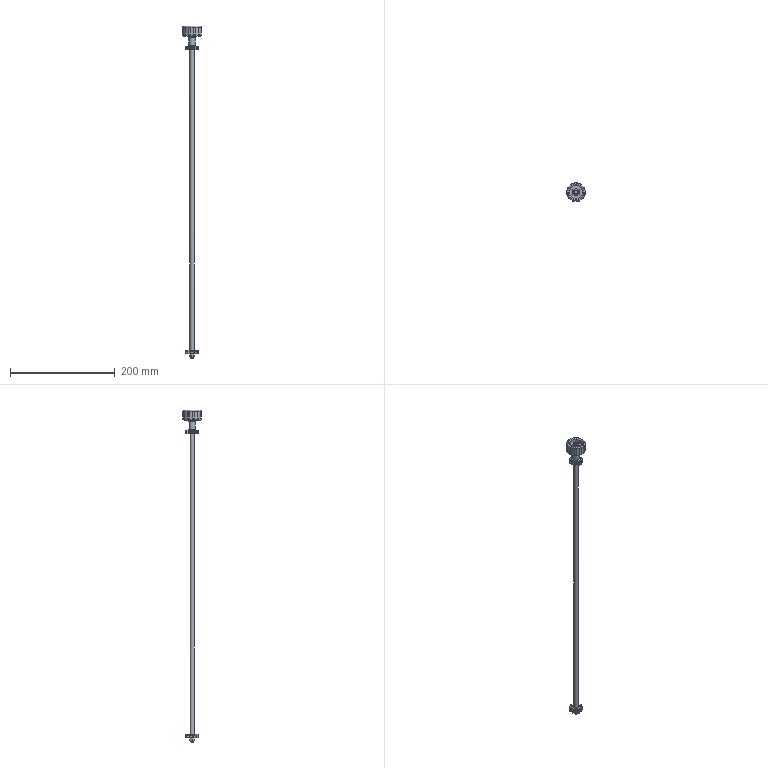Part | STEP file | DEWALT-DWE7294-B2-35 | 1 solid | 469 faces | box 36.143 x 35.85 x 635.164 mm | volume 52230 mm3 | cylinder 267 | plane 89 | torus 57 | spline 44 | sphere 12 | commonest cylinder face diameters 1.4 x166 1 x62 25 x23 36.2 x11 8 x2 5.415 x1